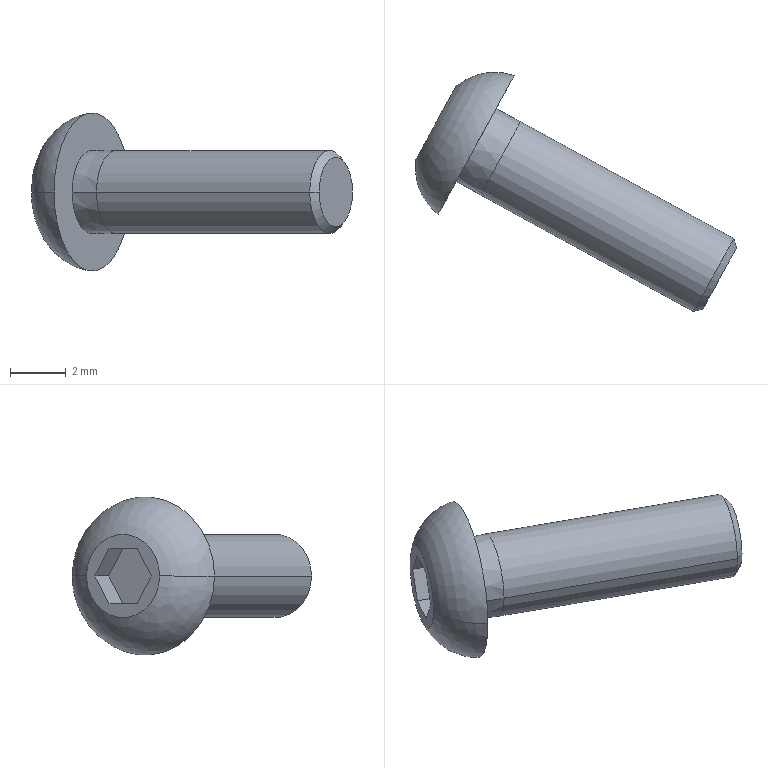Part | SolidWorks | features BaseBody 1 | 1 solid | 18 faces | box 11.561 x 8.617 x 5.7 mm | volume 97.979 mm3 | plane 10 | cone 4 | spline 2 | cylinder 2 | commonest cylinder face diameters 3 x2
STEP:
#1=CARTESIAN_POINT('',(472.21,-41.771,300.794));
#2=VERTEX_POINT('',#1);
#3=CARTESIAN_POINT('',(469.474,-46.771,300.794));
#4=VERTEX_POINT('',#3);
#5=CARTESIAN_POINT('',(470.842,-44.271,300.794));
#6=DIRECTION('',(0.8773,-0.4799,-0.000000008));
#7=DIRECTION('',(0.4799,0.8773,0.));
#8=AXIS2_PLACEMENT_3D('',#5,#6,#7);
#9=CIRCLE('',#8,2.85);
#10=EDGE_CURVE('',#2,#4,#9,.T.);
#11=ORIENTED_EDGE('',*,*,#10,.F.);
#12=CARTESIAN_POINT('',(470.115,-42.163,300.794));
#13=VERTEX_POINT('',#12);
#14=CARTESIAN_POINT('',(471.501,-43.777,300.794));
#15=DIRECTION('',(0.000000004,-0.000000009,1.));
#16=DIRECTION('',(0.4799,0.8773,0.000000006));
#17=AXIS2_PLACEMENT_3D('',#14,#15,#16);
#18=CIRCLE('',#17,2.127);
#19=EDGE_CURVE('',#2,#13,#18,.T.);
#20=ORIENTED_EDGE('',*,*,#19,.T.);
#21=CARTESIAN_POINT('',(468.675,-44.795,300.794));
#22=VERTEX_POINT('',#21);
#23=CARTESIAN_POINT('',(469.395,-43.479,300.794));
#24=DIRECTION('',(0.8773,-0.4799,-0.000000008));
#25=DIRECTION('',(0.4799,0.8773,0.));
#26=AXIS2_PLACEMENT_3D('',#23,#24,#25);
#27=CIRCLE('',#26,1.5);
#28=EDGE_CURVE('',#13,#22,#27,.T.);
#29=ORIENTED_EDGE('',*,*,#28,.T.);
#30=CARTESIAN_POINT('',(470.781,-45.093,300.794));
#31=DIRECTION('',(-0.000000004,0.000000009,-1.));
#32=DIRECTION('',(-0.4799,-0.8773,-0.000000006));
#33=AXIS2_PLACEMENT_3D('',#30,#31,#32);
#34=CIRCLE('',#33,2.127);
#35=EDGE_CURVE('',#4,#22,#34,.T.);
#36=ORIENTED_EDGE('',*,*,#35,.F.);
#37=EDGE_LOOP('',(#11,#20,#29,#36));
#38=FACE_OUTER_BOUND('',#37,.T.);
#39=CARTESIAN_POINT('',(472.21,-41.771,300.794));
#40=CARTESIAN_POINT('',(472.21,-41.771,302.464));
#41=CARTESIAN_POINT('',(471.643,-42.806,303.644));
#42=CARTESIAN_POINT('',(470.842,-44.271,303.644));
#43=CARTESIAN_POINT('',(470.041,-45.736,303.644));
#44=CARTESIAN_POINT('',(469.474,-46.771,302.464));
#45=CARTESIAN_POINT('',(469.474,-46.771,300.794));
#46=CARTESIAN_POINT('',(471.474,-41.511,300.794));
#47=CARTESIAN_POINT('',(471.474,-41.511,302.39));
#48=CARTESIAN_POINT('',(470.932,-42.501,303.519));
#49=CARTESIAN_POINT('',(470.166,-43.901,303.519));
#50=CARTESIAN_POINT('',(469.4,-45.302,303.519));
#51=CARTESIAN_POINT('',(468.858,-46.292,302.39));
#52=CARTESIAN_POINT('',(468.858,-46.292,300.794));
#53=CARTESIAN_POINT('',(470.707,-41.654,300.794));
#54=CARTESIAN_POINT('',(470.707,-41.654,302.101));
#55=CARTESIAN_POINT('',(470.263,-42.465,303.025));
#56=CARTESIAN_POINT('',(469.636,-43.611,303.025));
#57=CARTESIAN_POINT('',(469.009,-44.758,303.025));
#58=CARTESIAN_POINT('',(468.566,-45.568,302.101));
#59=CARTESIAN_POINT('',(468.566,-45.568,300.794));
#60=CARTESIAN_POINT('',(470.115,-42.163,300.794));
#61=CARTESIAN_POINT('',(470.115,-42.163,301.673));
#62=CARTESIAN_POINT('',(469.816,-42.708,302.294));
#63=CARTESIAN_POINT('',(469.395,-43.479,302.294));
#64=CARTESIAN_POINT('',(468.973,-44.25,302.294));
#65=CARTESIAN_POINT('',(468.675,-44.795,301.673));
#66=CARTESIAN_POINT('',(468.675,-44.795,300.794));
#67=(BOUNDED_SURFACE()B_SPLINE_SURFACE(3,3,((#39,#40,#41,#42,#43,#44,#45),(#46,#47,#48,#49,#50,#51,#52),(#53,#54,#55,#56,#57,#58,#59),(#60,#61,#62,#63,#64,#65,#66)),.UNSPECIFIED.,.F.,.F.,.T.)B_SPLINE_SURFACE_WITH_KNOTS((4,4),(4,3,4),(0.,1.),(0.,0.5,1.),.UNSPECIFIED.)GEOMETRIC_REPRESENTATION_ITEM()RATIONAL_B_SPLINE_SURFACE(((1.,0.8047,0.8047,1.,0.8047,0.8047,1.),(0.9103,0.7325,0.7325,0.9103,0.7325,0.7325,0.9103),(0.9103,0.7325,0.7325,0.9103,0.7325,0.7325,0.9103),(1.,0.8047,0.8047,1.,0.8047,0.8047,1.)))REPRESENTATION_ITEM('')SURFACE());
#68=ADVANCED_FACE('',(#38),#67,.T.);
#69=CARTESIAN_POINT('',(472.439,-43.435,300.794));
#70=VERTEX_POINT('',#69);
#71=CARTESIAN_POINT('',(471.,-46.067,300.794));
#72=VERTEX_POINT('',#71);
#73=CARTESIAN_POINT('',(471.72,-44.751,300.794));
#74=DIRECTION('',(0.8773,-0.4799,-0.000000008));
#75=DIRECTION('',(0.4799,0.8773,0.));
#76=AXIS2_PLACEMENT_3D('',#73,#74,#75);
#77=CIRCLE('',#76,1.5);
#78=EDGE_CURVE('',#70,#72,#77,.T.);
#79=ORIENTED_EDGE('',*,*,#78,.T.);
#80=CARTESIAN_POINT('',(478.676,-50.266,300.794));
#81=VERTEX_POINT('',#80);
#82=CARTESIAN_POINT('',(474.838,-48.166,300.794));
#83=DIRECTION('',(0.8773,-0.4799,-0.000000008));
#84=VECTOR('',#83,1000.);
#85=LINE('',#82,#84);
#86=EDGE_CURVE('',#72,#81,#85,.T.);
#87=ORIENTED_EDGE('',*,*,#86,.T.);
#88=CARTESIAN_POINT('',(480.116,-47.634,300.794));
#89=VERTEX_POINT('',#88);
#90=CARTESIAN_POINT('',(479.396,-48.95,300.794));
#91=DIRECTION('',(-0.8773,0.4799,0.000000008));
#92=DIRECTION('',(0.4799,0.8773,0.));
#93=AXIS2_PLACEMENT_3D('',#90,#91,#92);
#94=CIRCLE('',#93,1.5);
#95=EDGE_CURVE('',#81,#89,#94,.T.);
#96=ORIENTED_EDGE('',*,*,#95,.T.);
#97=CARTESIAN_POINT('',(476.278,-45.535,300.794));
#98=DIRECTION('',(0.8773,-0.4799,-0.000000008));
#99=VECTOR('',#98,1000.);
#100=LINE('',#97,#99);
#101=EDGE_CURVE('',#70,#89,#100,.T.);
#102=ORIENTED_EDGE('',*,*,#101,.F.);
#103=EDGE_LOOP('',(#79,#87,#96,#102));
#104=FACE_OUTER_BOUND('',#103,.T.);
#105=CARTESIAN_POINT('',(475.558,-46.851,300.794));
#106=DIRECTION('',(0.8773,-0.4799,-0.000000008));
#107=DIRECTION('',(0.4799,0.8773,0.));
#108=AXIS2_PLACEMENT_3D('',#105,#106,#107);
#109=CYLINDRICAL_SURFACE('',#108,1.5);
#110=ADVANCED_FACE('',(#104),#109,.T.);
#111=CARTESIAN_POINT('',(471.562,-42.956,300.794));
#112=VERTEX_POINT('',#111);
#113=CARTESIAN_POINT('',(470.123,-45.586,300.794));
#114=VERTEX_POINT('',#113);
#115=CARTESIAN_POINT('',(470.842,-44.271,300.794));
#116=DIRECTION('',(0.8773,-0.4799,-0.000000008));
#117=DIRECTION('',(0.4799,0.8773,0.));
#118=AXIS2_PLACEMENT_3D('',#115,#116,#117);
#119=CIRCLE('',#118,1.499);
#120=EDGE_CURVE('',#112,#114,#119,.T.);
#121=ORIENTED_EDGE('',*,*,#120,.T.);
#122=CARTESIAN_POINT('',(471.,-46.067,300.794));
#123=DIRECTION('',(0.877,-0.4806,-0.000000008));
#124=VECTOR('',#123,1000.);
#125=LINE('',#122,#124);
#126=EDGE_CURVE('',#114,#72,#125,.T.);
#127=ORIENTED_EDGE('',*,*,#126,.T.);
#128=ORIENTED_EDGE('',*,*,#78,.F.);
#129=CARTESIAN_POINT('',(472.439,-43.435,300.794));
#130=DIRECTION('',(0.8777,-0.4793,-0.000000008));
#131=VECTOR('',#130,1000.);
#132=LINE('',#129,#131);
#133=EDGE_CURVE('',#112,#70,#132,.T.);
#134=ORIENTED_EDGE('',*,*,#133,.F.);
#135=EDGE_LOOP('',(#121,#127,#128,#134));
#136=FACE_OUTER_BOUND('',#135,.T.);
#137=CARTESIAN_POINT('',(471.72,-44.751,300.794));
#138=DIRECTION('',(0.8773,-0.4799,-0.000000008));
#139=DIRECTION('',(0.4799,0.8773,0.));
#140=AXIS2_PLACEMENT_3D('',#137,#138,#139);
#141=CONICAL_SURFACE('',#140,1.5,0.00075);
#142=ADVANCED_FACE('',(#136),#141,.T.);
#143=CARTESIAN_POINT('',(479.016,-50.167,300.794));
#144=VERTEX_POINT('',#143);
#145=CARTESIAN_POINT('',(480.215,-47.973,300.794));
#146=VERTEX_POINT('',#145);
#147=CARTESIAN_POINT('',(479.615,-49.07,300.794));
#148=DIRECTION('',(-0.8773,0.4799,0.000000008));
#149=DIRECTION('',(-0.4799,-0.8773,0.));
#150=AXIS2_PLACEMENT_3D('',#147,#148,#149);
#151=CIRCLE('',#150,1.25);
#152=EDGE_CURVE('',#144,#146,#151,.T.);
#153=ORIENTED_EDGE('',*,*,#152,.T.);
#154=CARTESIAN_POINT('',(480.116,-47.634,300.794));
#155=DIRECTION('',(-0.281,0.9597,0.000000005));
#156=VECTOR('',#155,1000.);
#157=LINE('',#154,#156);
#158=EDGE_CURVE('',#146,#89,#157,.T.);
#159=ORIENTED_EDGE('',*,*,#158,.T.);
#160=ORIENTED_EDGE('',*,*,#95,.F.);
#161=CARTESIAN_POINT('',(478.676,-50.266,300.794));
#162=DIRECTION('',(-0.9597,-0.281,0.000000005));
#163=VECTOR('',#162,1000.);
#164=LINE('',#161,#163);
#165=EDGE_CURVE('',#144,#81,#164,.T.);
#166=ORIENTED_EDGE('',*,*,#165,.F.);
#167=EDGE_LOOP('',(#153,#159,#160,#166));
#168=FACE_OUTER_BOUND('',#167,.T.);
#169=CARTESIAN_POINT('',(479.396,-48.95,300.794));
#170=DIRECTION('',(-0.8773,0.4799,0.000000008));
#171=DIRECTION('',(-0.4799,-0.8773,0.));
#172=AXIS2_PLACEMENT_3D('',#169,#170,#171);
#173=CONICAL_SURFACE('',#172,1.5,0.7854);
#174=ADVANCED_FACE('',(#168),#173,.T.);
#175=ORIENTED_EDGE('',*,*,#86,.F.);
#176=CARTESIAN_POINT('',(471.72,-44.751,300.794));
#177=DIRECTION('',(0.8773,-0.4799,-0.000000008));
#178=DIRECTION('',(0.4799,0.8773,0.));
#179=AXIS2_PLACEMENT_3D('',#176,#177,#178);
#180=CIRCLE('',#179,1.5);
#181=EDGE_CURVE('',#72,#70,#180,.T.);
#182=ORIENTED_EDGE('',*,*,#181,.T.);
#183=ORIENTED_EDGE('',*,*,#101,.T.);
#184=CARTESIAN_POINT('',(479.396,-48.95,300.794));
#185=DIRECTION('',(-0.8773,0.4799,0.000000008));
#186=DIRECTION('',(0.4799,0.8773,0.));
#187=AXIS2_PLACEMENT_3D('',#184,#185,#186);
#188=CIRCLE('',#187,1.5);
#189=EDGE_CURVE('',#89,#81,#188,.T.);
#190=ORIENTED_EDGE('',*,*,#189,.T.);
#191=EDGE_LOOP('',(#175,#182,#183,#190));
#192=FACE_OUTER_BOUND('',#191,.T.);
#193=CARTESIAN_POINT('',(475.558,-46.851,300.794));
#194=DIRECTION('',(0.8773,-0.4799,-0.000000008));
#195=DIRECTION('',(0.4799,0.8773,0.));
#196=AXIS2_PLACEMENT_3D('',#193,#194,#195);
#197=CYLINDRICAL_SURFACE('',#196,1.5);
#198=ADVANCED_FACE('',(#192),#197,.T.);
#199=ORIENTED_EDGE('',*,*,#126,.F.);
#200=CARTESIAN_POINT('',(470.842,-44.271,300.794));
#201=DIRECTION('',(0.8773,-0.4799,-0.000000008));
#202=DIRECTION('',(0.4799,0.8773,0.));
#203=AXIS2_PLACEMENT_3D('',#200,#201,#202);
#204=CIRCLE('',#203,1.499);
#205=EDGE_CURVE('',#114,#112,#204,.T.);
#206=ORIENTED_EDGE('',*,*,#205,.T.);
#207=ORIENTED_EDGE('',*,*,#133,.T.);
#208=ORIENTED_EDGE('',*,*,#181,.F.);
#209=EDGE_LOOP('',(#199,#206,#207,#208));
#210=FACE_OUTER_BOUND('',#209,.T.);
#211=CARTESIAN_POINT('',(471.72,-44.751,300.794));
#212=DIRECTION('',(0.8773,-0.4799,-0.000000008));
#213=DIRECTION('',(0.4799,0.8773,0.));
#214=AXIS2_PLACEMENT_3D('',#211,#212,#213);
#215=CONICAL_SURFACE('',#214,1.5,0.00075);
#216=ADVANCED_FACE('',(#210),#215,.T.);
#217=ORIENTED_EDGE('',*,*,#158,.F.);
#218=CARTESIAN_POINT('',(479.615,-49.07,300.794));
#219=DIRECTION('',(-0.8773,0.4799,0.000000008));
#220=DIRECTION('',(-0.4799,-0.8773,0.));
#221=AXIS2_PLACEMENT_3D('',#218,#219,#220);
#222=CIRCLE('',#221,1.25);
#223=EDGE_CURVE('',#146,#144,#222,.T.);
#224=ORIENTED_EDGE('',*,*,#223,.T.);
#225=ORIENTED_EDGE('',*,*,#165,.T.);
#226=ORIENTED_EDGE('',*,*,#189,.F.);
#227=EDGE_LOOP('',(#217,#224,#225,#226));
#228=FACE_OUTER_BOUND('',#227,.T.);
#229=CARTESIAN_POINT('',(479.396,-48.95,300.794));
#230=DIRECTION('',(-0.8773,0.4799,0.000000008));
#231=DIRECTION('',(-0.4799,-0.8773,0.));
#232=AXIS2_PLACEMENT_3D('',#229,#230,#231);
#233=CONICAL_SURFACE('',#232,1.5,0.7854);
#234=ADVANCED_FACE('',(#228),#233,.T.);
#235=ORIENTED_EDGE('',*,*,#120,.F.);
#236=ORIENTED_EDGE('',*,*,#205,.F.);
#237=EDGE_LOOP('',(#235,#236));
#238=FACE_BOUND('',#237,.T.);
#239=CARTESIAN_POINT('',(470.842,-44.271,300.794));
#240=DIRECTION('',(0.8773,-0.4799,-0.000000008));
#241=DIRECTION('',(0.4799,0.8773,0.));
#242=AXIS2_PLACEMENT_3D('',#239,#240,#241);
#243=CIRCLE('',#242,2.85);
#244=EDGE_CURVE('',#4,#2,#243,.T.);
#245=ORIENTED_EDGE('',*,*,#244,.T.);
#246=ORIENTED_EDGE('',*,*,#10,.T.);
#247=EDGE_LOOP('',(#245,#246));
#248=FACE_OUTER_BOUND('',#247,.T.);
#249=CARTESIAN_POINT('',(470.158,-45.521,300.794));
#250=DIRECTION('',(0.8773,-0.4799,-0.000000008));
#251=DIRECTION('',(0.4799,0.8773,0.));
#252=AXIS2_PLACEMENT_3D('',#249,#250,#251);
#253=PLANE('',#252);
#254=ADVANCED_FACE('',(#238,#248),#253,.T.);
#255=ORIENTED_EDGE('',*,*,#152,.F.);
#256=ORIENTED_EDGE('',*,*,#223,.F.);
#257=EDGE_LOOP('',(#255,#256));
#258=FACE_OUTER_BOUND('',#257,.T.);
#259=CARTESIAN_POINT('',(479.315,-49.618,300.794));
#260=DIRECTION('',(0.8773,-0.4799,-0.000000008));
#261=DIRECTION('',(0.4799,0.8773,0.));
#262=AXIS2_PLACEMENT_3D('',#259,#260,#261);
#263=PLANE('',#262);
#264=ADVANCED_FACE('',(#258),#263,.T.);
#265=ORIENTED_EDGE('',*,*,#19,.F.);
#266=ORIENTED_EDGE('',*,*,#244,.F.);
#267=ORIENTED_EDGE('',*,*,#35,.T.);
#268=CARTESIAN_POINT('',(469.395,-43.479,300.794));
#269=DIRECTION('',(0.8773,-0.4799,-0.000000008));
#270=DIRECTION('',(0.4799,0.8773,0.));
#271=AXIS2_PLACEMENT_3D('',#268,#269,#270);
#272=CIRCLE('',#271,1.5);
#273=EDGE_CURVE('',#22,#13,#272,.T.);
#274=ORIENTED_EDGE('',*,*,#273,.T.);
#275=EDGE_LOOP('',(#265,#266,#267,#274));
#276=FACE_OUTER_BOUND('',#275,.T.);
#277=CARTESIAN_POINT('',(469.474,-46.771,300.794));
#278=CARTESIAN_POINT('',(469.474,-46.771,295.094));
#279=CARTESIAN_POINT('',(472.21,-41.771,295.094));
#280=CARTESIAN_POINT('',(472.21,-41.771,300.794));
#281=CARTESIAN_POINT('',(468.858,-46.292,300.794));
#282=CARTESIAN_POINT('',(468.858,-46.292,295.344));
#283=CARTESIAN_POINT('',(471.474,-41.511,295.344));
#284=CARTESIAN_POINT('',(471.474,-41.511,300.794));
#285=CARTESIAN_POINT('',(468.566,-45.568,300.794));
#286=CARTESIAN_POINT('',(468.566,-45.568,296.333));
#287=CARTESIAN_POINT('',(470.707,-41.654,296.333));
#288=CARTESIAN_POINT('',(470.707,-41.654,300.794));
#289=CARTESIAN_POINT('',(468.675,-44.795,300.794));
#290=CARTESIAN_POINT('',(468.675,-44.795,297.794));
#291=CARTESIAN_POINT('',(470.115,-42.163,297.794));
#292=CARTESIAN_POINT('',(470.115,-42.163,300.794));
#293=(BOUNDED_SURFACE()B_SPLINE_SURFACE(3,3,((#277,#278,#279,#280),(#281,#282,#283,#284),(#285,#286,#287,#288),(#289,#290,#291,#292)),.UNSPECIFIED.,.F.,.F.,.T.)B_SPLINE_SURFACE_WITH_KNOTS((4,4),(4,4),(0.,1.),(0.,1.),.UNSPECIFIED.)GEOMETRIC_REPRESENTATION_ITEM()RATIONAL_B_SPLINE_SURFACE(((1.,0.3333,0.3333,1.),(0.9103,0.3034,0.3034,0.9103),(0.9103,0.3034,0.3034,0.9103),(1.,0.3333,0.3333,1.)))REPRESENTATION_ITEM('')SURFACE());
#294=ADVANCED_FACE('',(#276),#293,.T.);
#295=ORIENTED_EDGE('',*,*,#273,.F.);
#296=ORIENTED_EDGE('',*,*,#28,.F.);
#297=EDGE_LOOP('',(#295,#296));
#298=FACE_OUTER_BOUND('',#297,.T.);
#299=CARTESIAN_POINT('',(469.672,-42.973,299.794));
#300=VERTEX_POINT('',#299);
#301=CARTESIAN_POINT('',(469.949,-42.466,300.794));
#302=VERTEX_POINT('',#301);
#303=CARTESIAN_POINT('',(469.672,-42.973,299.794));
#304=DIRECTION('',(0.24,0.4387,0.866));
#305=VECTOR('',#304,1000.);
#306=LINE('',#303,#305);
#307=EDGE_CURVE('',#300,#302,#306,.T.);
#308=ORIENTED_EDGE('',*,*,#307,.T.);
#309=CARTESIAN_POINT('',(469.672,-42.973,301.794));
#310=VERTEX_POINT('',#309);
#311=CARTESIAN_POINT('',(469.949,-42.466,300.794));
#312=DIRECTION('',(-0.24,-0.4387,0.866));
#313=VECTOR('',#312,1000.);
#314=LINE('',#311,#313);
#315=EDGE_CURVE('',#302,#310,#314,.T.);
#316=ORIENTED_EDGE('',*,*,#315,.T.);
#317=CARTESIAN_POINT('',(469.118,-43.986,301.794));
#318=VERTEX_POINT('',#317);
#319=CARTESIAN_POINT('',(469.035,-44.137,301.794));
#320=DIRECTION('',(-0.4799,-0.8773,0.));
#321=VECTOR('',#320,1000.);
#322=LINE('',#319,#321);
#323=EDGE_CURVE('',#310,#318,#322,.T.);
#324=ORIENTED_EDGE('',*,*,#323,.T.);
#325=CARTESIAN_POINT('',(468.841,-44.492,300.794));
#326=VERTEX_POINT('',#325);
#327=CARTESIAN_POINT('',(469.118,-43.986,301.794));
#328=DIRECTION('',(-0.24,-0.4387,-0.866));
#329=VECTOR('',#328,1000.);
#330=LINE('',#327,#329);
#331=EDGE_CURVE('',#318,#326,#330,.T.);
#332=ORIENTED_EDGE('',*,*,#331,.T.);
#333=CARTESIAN_POINT('',(469.118,-43.986,299.794));
#334=VERTEX_POINT('',#333);
#335=CARTESIAN_POINT('',(468.841,-44.492,300.794));
#336=DIRECTION('',(0.24,0.4387,-0.866));
#337=VECTOR('',#336,1000.);
#338=LINE('',#335,#337);
#339=EDGE_CURVE('',#326,#334,#338,.T.);
#340=ORIENTED_EDGE('',*,*,#339,.T.);
#341=CARTESIAN_POINT('',(469.035,-44.137,299.794));
#342=DIRECTION('',(0.4799,0.8773,0.));
#343=VECTOR('',#342,1000.);
#344=LINE('',#341,#343);
#345=EDGE_CURVE('',#334,#300,#344,.T.);
#346=ORIENTED_EDGE('',*,*,#345,.T.);
#347=EDGE_LOOP('',(#308,#316,#324,#332,#340,#346));
#348=FACE_BOUND('',#347,.T.);
#349=CARTESIAN_POINT('',(469.035,-44.137,300.794));
#350=DIRECTION('',(-0.8773,0.4799,0.000000008));
#351=DIRECTION('',(-0.4799,-0.8773,0.));
#352=AXIS2_PLACEMENT_3D('',#349,#350,#351);
#353=PLANE('',#352);
#354=ADVANCED_FACE('',(#298,#348),#353,.T.);
#355=CARTESIAN_POINT('',(470.584,-43.472,301.794));
#356=VERTEX_POINT('',#355);
#357=CARTESIAN_POINT('',(469.672,-42.973,301.794));
#358=DIRECTION('',(0.8773,-0.4799,-0.000000008));
#359=VECTOR('',#358,1000.);
#360=LINE('',#357,#359);
#361=EDGE_CURVE('',#310,#356,#360,.T.);
#362=ORIENTED_EDGE('',*,*,#361,.F.);
#363=ORIENTED_EDGE('',*,*,#315,.F.);
#364=CARTESIAN_POINT('',(470.861,-42.965,300.794));
#365=VERTEX_POINT('',#364);
#366=CARTESIAN_POINT('',(470.861,-42.965,300.794));
#367=DIRECTION('',(-0.8773,0.4799,0.000000008));
#368=VECTOR('',#367,1000.);
#369=LINE('',#366,#368);
#370=EDGE_CURVE('',#365,#302,#369,.T.);
#371=ORIENTED_EDGE('',*,*,#370,.F.);
#372=CARTESIAN_POINT('',(470.584,-43.472,301.794));
#373=DIRECTION('',(0.24,0.4387,-0.866));
#374=VECTOR('',#373,1000.);
#375=LINE('',#372,#374);
#376=EDGE_CURVE('',#356,#365,#375,.T.);
#377=ORIENTED_EDGE('',*,*,#376,.F.);
#378=EDGE_LOOP('',(#362,#363,#371,#377));
#379=FACE_OUTER_BOUND('',#378,.T.);
#380=CARTESIAN_POINT('',(469.672,-42.973,301.794));
#381=DIRECTION('',(0.4156,0.7598,0.5));
#382=DIRECTION('',(0.,-0.5497,0.8353));
#383=AXIS2_PLACEMENT_3D('',#380,#381,#382);
#384=PLANE('',#383);
#385=ADVANCED_FACE('',(#379),#384,.F.);
#386=ORIENTED_EDGE('',*,*,#370,.T.);
#387=ORIENTED_EDGE('',*,*,#307,.F.);
#388=CARTESIAN_POINT('',(470.584,-43.472,299.794));
#389=VERTEX_POINT('',#388);
#390=CARTESIAN_POINT('',(470.584,-43.472,299.794));
#391=DIRECTION('',(-0.8773,0.4799,0.000000008));
#392=VECTOR('',#391,1000.);
#393=LINE('',#390,#392);
#394=EDGE_CURVE('',#389,#300,#393,.T.);
#395=ORIENTED_EDGE('',*,*,#394,.F.);
#396=CARTESIAN_POINT('',(470.861,-42.965,300.794));
#397=DIRECTION('',(-0.24,-0.4387,-0.866));
#398=VECTOR('',#397,1000.);
#399=LINE('',#396,#398);
#400=EDGE_CURVE('',#365,#389,#399,.T.);
#401=ORIENTED_EDGE('',*,*,#400,.F.);
#402=EDGE_LOOP('',(#386,#387,#395,#401));
#403=FACE_OUTER_BOUND('',#402,.T.);
#404=CARTESIAN_POINT('',(469.949,-42.466,300.794));
#405=DIRECTION('',(0.4156,0.7598,-0.5));
#406=DIRECTION('',(0.,0.5497,0.8353));
#407=AXIS2_PLACEMENT_3D('',#404,#405,#406);
#408=PLANE('',#407);
#409=ADVANCED_FACE('',(#403),#408,.F.);
#410=ORIENTED_EDGE('',*,*,#394,.T.);
#411=ORIENTED_EDGE('',*,*,#345,.F.);
#412=CARTESIAN_POINT('',(470.03,-44.485,299.794));
#413=VERTEX_POINT('',#412);
#414=CARTESIAN_POINT('',(470.03,-44.485,299.794));
#415=DIRECTION('',(-0.8773,0.4799,0.000000008));
#416=VECTOR('',#415,1000.);
#417=LINE('',#414,#416);
#418=EDGE_CURVE('',#413,#334,#417,.T.);
#419=ORIENTED_EDGE('',*,*,#418,.F.);
#420=CARTESIAN_POINT('',(470.584,-43.472,299.794));
#421=DIRECTION('',(-0.4799,-0.8773,-0.000000006));
#422=VECTOR('',#421,1000.);
#423=LINE('',#420,#422);
#424=EDGE_CURVE('',#389,#413,#423,.T.);
#425=ORIENTED_EDGE('',*,*,#424,.F.);
#426=EDGE_LOOP('',(#410,#411,#419,#425));
#427=FACE_OUTER_BOUND('',#426,.T.);
#428=CARTESIAN_POINT('',(469.672,-42.973,299.794));
#429=DIRECTION('',(-0.000000004,0.000000009,-1.));
#430=DIRECTION('',(0.,1.,0.000000009));
#431=AXIS2_PLACEMENT_3D('',#428,#429,#430);
#432=PLANE('',#431);
#433=ADVANCED_FACE('',(#427),#432,.F.);
#434=ORIENTED_EDGE('',*,*,#418,.T.);
#435=ORIENTED_EDGE('',*,*,#339,.F.);
#436=CARTESIAN_POINT('',(469.753,-44.991,300.794));
#437=VERTEX_POINT('',#436);
#438=CARTESIAN_POINT('',(469.753,-44.991,300.794));
#439=DIRECTION('',(-0.8773,0.4799,0.000000008));
#440=VECTOR('',#439,1000.);
#441=LINE('',#438,#440);
#442=EDGE_CURVE('',#437,#326,#441,.T.);
#443=ORIENTED_EDGE('',*,*,#442,.F.);
#444=CARTESIAN_POINT('',(470.03,-44.485,299.794));
#445=DIRECTION('',(-0.24,-0.4387,0.866));
#446=VECTOR('',#445,1000.);
#447=LINE('',#444,#446);
#448=EDGE_CURVE('',#413,#437,#447,.T.);
#449=ORIENTED_EDGE('',*,*,#448,.F.);
#450=EDGE_LOOP('',(#434,#435,#443,#449));
#451=FACE_OUTER_BOUND('',#450,.T.);
#452=CARTESIAN_POINT('',(469.118,-43.986,299.794));
#453=DIRECTION('',(-0.4156,-0.7598,-0.5));
#454=DIRECTION('',(0.,0.5497,-0.8353));
#455=AXIS2_PLACEMENT_3D('',#452,#453,#454);
#456=PLANE('',#455);
#457=ADVANCED_FACE('',(#451),#456,.F.);
#458=ORIENTED_EDGE('',*,*,#442,.T.);
#459=ORIENTED_EDGE('',*,*,#331,.F.);
#460=CARTESIAN_POINT('',(470.03,-44.485,301.794));
#461=VERTEX_POINT('',#460);
#462=CARTESIAN_POINT('',(470.03,-44.485,301.794));
#463=DIRECTION('',(-0.8773,0.4799,0.000000008));
#464=VECTOR('',#463,1000.);
#465=LINE('',#462,#464);
#466=EDGE_CURVE('',#461,#318,#465,.T.);
#467=ORIENTED_EDGE('',*,*,#466,.F.);
#468=CARTESIAN_POINT('',(469.753,-44.991,300.794));
#469=DIRECTION('',(0.24,0.4387,0.866));
#470=VECTOR('',#469,1000.);
#471=LINE('',#468,#470);
#472=EDGE_CURVE('',#437,#461,#471,.T.);
#473=ORIENTED_EDGE('',*,*,#472,.F.);
#474=EDGE_LOOP('',(#458,#459,#467,#473));
#475=FACE_OUTER_BOUND('',#474,.T.);
#476=CARTESIAN_POINT('',(468.841,-44.492,300.794));
#477=DIRECTION('',(-0.4156,-0.7598,0.5));
#478=DIRECTION('',(0.,-0.5497,-0.8353));
#479=AXIS2_PLACEMENT_3D('',#476,#477,#478);
#480=PLANE('',#479);
#481=ADVANCED_FACE('',(#475),#480,.F.);
#482=ORIENTED_EDGE('',*,*,#466,.T.);
#483=ORIENTED_EDGE('',*,*,#323,.F.);
#484=ORIENTED_EDGE('',*,*,#361,.T.);
#485=CARTESIAN_POINT('',(470.03,-44.485,301.794));
#486=DIRECTION('',(0.4799,0.8773,0.000000006));
#487=VECTOR('',#486,1000.);
#488=LINE('',#485,#487);
#489=EDGE_CURVE('',#461,#356,#488,.T.);
#490=ORIENTED_EDGE('',*,*,#489,.F.);
#491=EDGE_LOOP('',(#482,#483,#484,#490));
#492=FACE_OUTER_BOUND('',#491,.T.);
#493=CARTESIAN_POINT('',(469.118,-43.986,301.794));
#494=DIRECTION('',(0.000000004,-0.000000009,1.));
#495=DIRECTION('',(0.,-1.,-0.000000009));
#496=AXIS2_PLACEMENT_3D('',#493,#494,#495);
#497=PLANE('',#496);
#498=ADVANCED_FACE('',(#492),#497,.F.);
#499=ORIENTED_EDGE('',*,*,#448,.T.);
#500=ORIENTED_EDGE('',*,*,#472,.T.);
#501=ORIENTED_EDGE('',*,*,#489,.T.);
#502=ORIENTED_EDGE('',*,*,#376,.T.);
#503=ORIENTED_EDGE('',*,*,#400,.T.);
#504=ORIENTED_EDGE('',*,*,#424,.T.);
#505=EDGE_LOOP('',(#499,#500,#501,#502,#503,#504));
#506=FACE_OUTER_BOUND('',#505,.T.);
#507=CARTESIAN_POINT('',(470.307,-43.978,300.794));
#508=DIRECTION('',(-0.8773,0.4799,0.000000008));
#509=DIRECTION('',(-0.4799,-0.8773,0.));
#510=AXIS2_PLACEMENT_3D('',#507,#508,#509);
#511=PLANE('',#510);
#512=ADVANCED_FACE('',(#506),#511,.T.);
#513=CLOSED_SHELL('',(#68,#110,#142,#174,#198,#216,#234,#254,#264,#294,#354,#385,#409,#433,#457,#481,#498,#512));
#514=MANIFOLD_SOLID_BREP('',#513);
#515=CARTESIAN_POINT('',(0.,0.,0.));
#516=DIRECTION('',(0.,0.,1.));
#517=DIRECTION('',(1.,0.,0.));
#518=AXIS2_PLACEMENT_3D('',#515,#516,#517);
#519=(LENGTH_UNIT()NAMED_UNIT(*)SI_UNIT(.MILLI.,.METRE.));
#520=UNCERTAINTY_MEASURE_WITH_UNIT(LENGTH_MEASURE(0.00001),#519,'','');
#521=(NAMED_UNIT(*)PLANE_ANGLE_UNIT()SI_UNIT($,.RADIAN.));
#522=(NAMED_UNIT(*)SI_UNIT($,.STERADIAN.)SOLID_ANGLE_UNIT());
#523=(GEOMETRIC_REPRESENTATION_CONTEXT(3)GLOBAL_UNCERTAINTY_ASSIGNED_CONTEXT((#520))GLOBAL_UNIT_ASSIGNED_CONTEXT((#519,#521,#522))REPRESENTATION_CONTEXT('',''));
#524=ADVANCED_BREP_SHAPE_REPRESENTATION('',(#514,#518),#523);